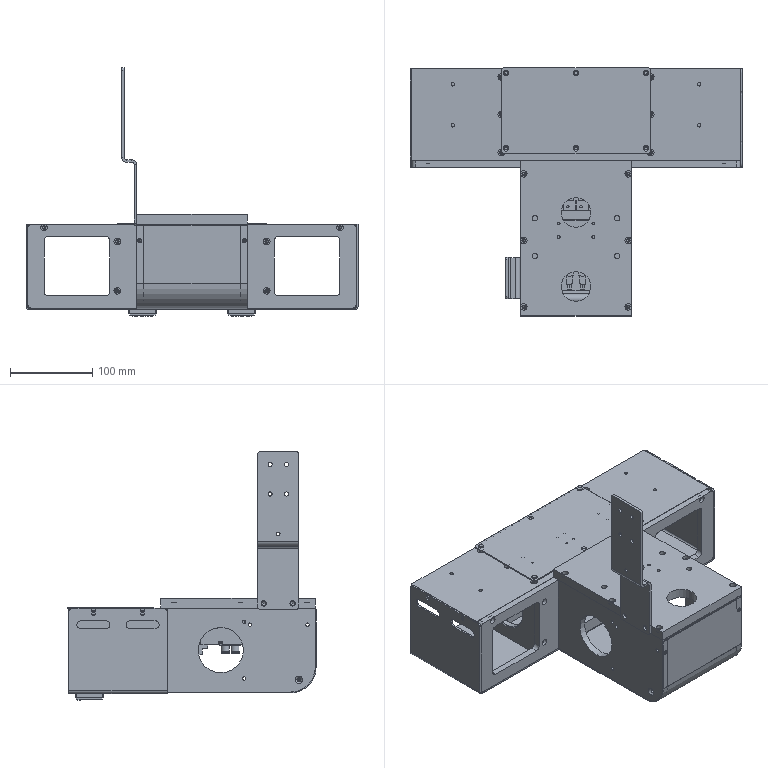Part | NX | 25 solids | 1842 faces | box 404 x 302 x 302.5 mm | volume 1808457 mm3 | plane 1046 | spline 360 | cylinder 330 | cone 106 | commonest cylinder face diameters 3.3 x50 4.5 x44 10 x32 2 x24 5 x20 2.5 x16